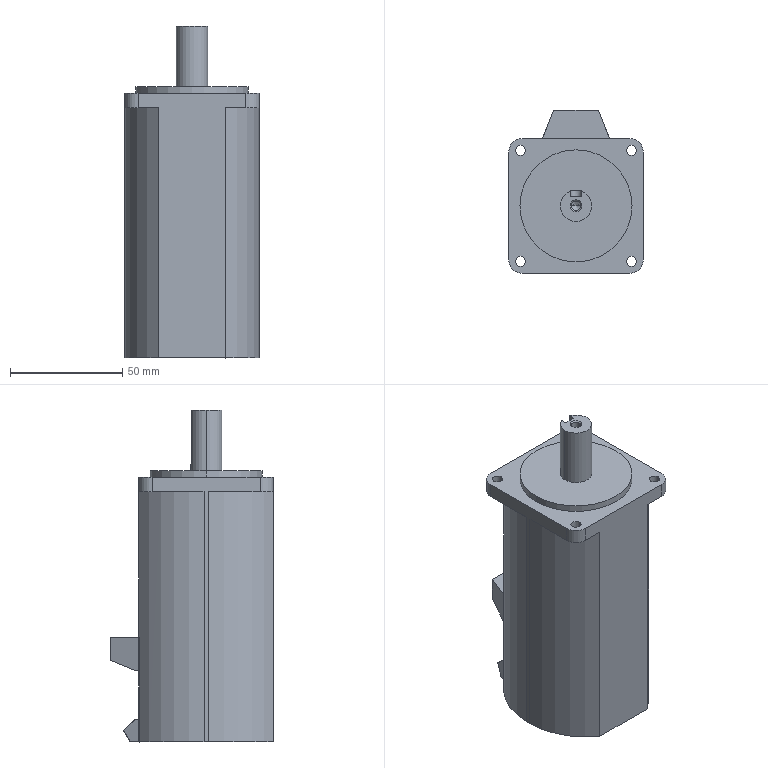Part | NX | 1 solid | 316 faces | box 60 x 72.701 x 148 mm | volume 381315 mm3 | plane 276 | cylinder 34 | cone 4 | sphere 2 | commonest cylinder face diameters 0.6 x11 4.5 x8 12 x4 71.067 x4 4.2 x2 14 x2